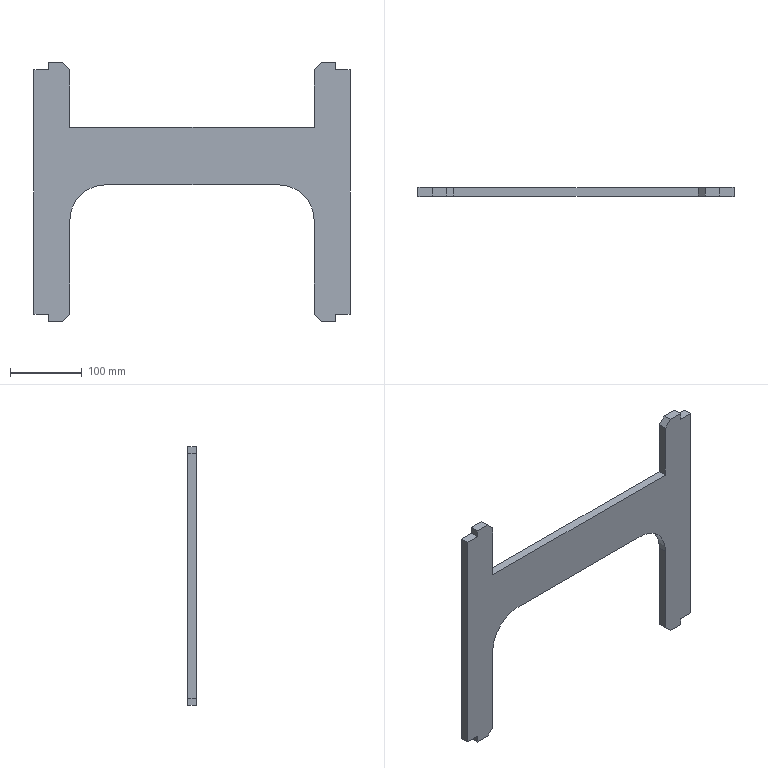Part | STEP file | MOTOR.RIB.stp | 1 solid | 30 faces | box 440 x 12 x 360 mm | volume 759276 mm3 | spline 14 | plane 12 | cylinder 4 | commonest cylinder face diameters 100 x4